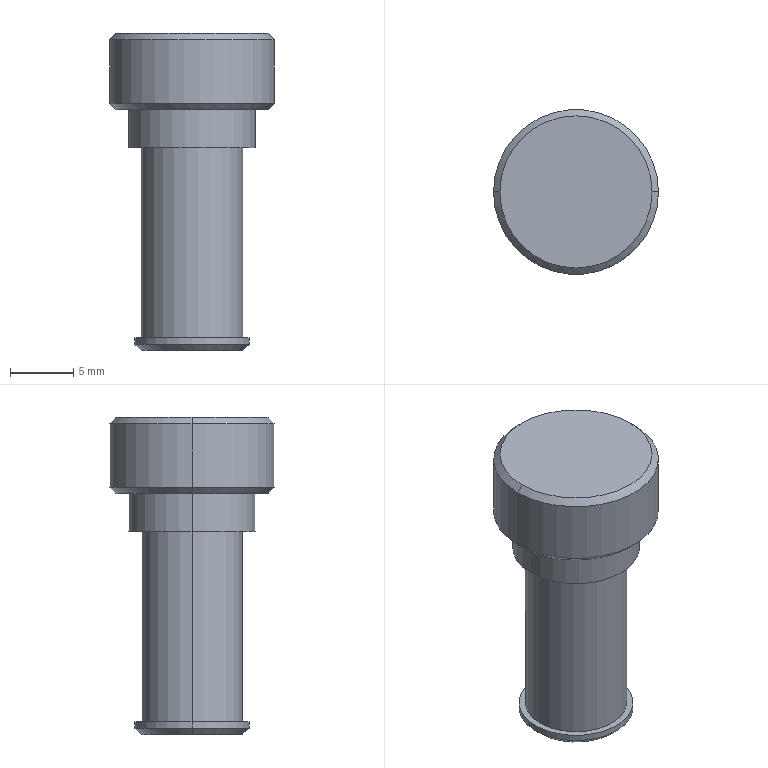Part | SolidWorks | features ICE 4, Chamfer 1, Extrusion 1 | 1 solid | 19 faces | box 13 x 13 x 25 mm | volume 1836 mm3 | cylinder 8 | cone 6 | plane 5 | commonest cylinder face diameters 8 x2 9 x2 10 x2 13 x2
STEP:
#1=CARTESIAN_POINT('',(-6.,0.,19.));
#2=VERTEX_POINT('',#1);
#3=CARTESIAN_POINT('',(6.,0.,19.));
#4=VERTEX_POINT('',#3);
#5=CARTESIAN_POINT('',(0.,0.,19.));
#6=DIRECTION('',(0.,0.,-1.));
#7=DIRECTION('',(1.,0.,0.));
#8=AXIS2_PLACEMENT_3D('',#5,#6,#7);
#9=CIRCLE('',#8,6.);
#10=EDGE_CURVE('',#2,#4,#9,.T.);
#11=ORIENTED_EDGE('',*,*,#10,.F.);
#12=CARTESIAN_POINT('',(-6.5,0.,19.5));
#13=VERTEX_POINT('',#12);
#14=CARTESIAN_POINT('',(-6.5,0.,19.5));
#15=DIRECTION('',(-0.7071,0.,0.7071));
#16=VECTOR('',#15,1000.);
#17=LINE('',#14,#16);
#18=EDGE_CURVE('',#2,#13,#17,.T.);
#19=ORIENTED_EDGE('',*,*,#18,.T.);
#20=CARTESIAN_POINT('',(6.5,0.,19.5));
#21=VERTEX_POINT('',#20);
#22=CARTESIAN_POINT('',(0.,0.,19.5));
#23=DIRECTION('',(0.,0.,1.));
#24=DIRECTION('',(1.,0.,0.));
#25=AXIS2_PLACEMENT_3D('',#22,#23,#24);
#26=CIRCLE('',#25,6.5);
#27=EDGE_CURVE('',#21,#13,#26,.T.);
#28=ORIENTED_EDGE('',*,*,#27,.F.);
#29=CARTESIAN_POINT('',(6.5,0.,19.5));
#30=DIRECTION('',(0.7071,0.,0.7071));
#31=VECTOR('',#30,1000.);
#32=LINE('',#29,#31);
#33=EDGE_CURVE('',#4,#21,#32,.T.);
#34=ORIENTED_EDGE('',*,*,#33,.F.);
#35=EDGE_LOOP('',(#11,#19,#28,#34));
#36=FACE_OUTER_BOUND('',#35,.T.);
#37=CARTESIAN_POINT('',(0.,0.,19.5));
#38=DIRECTION('',(0.,0.,1.));
#39=DIRECTION('',(1.,0.,0.));
#40=AXIS2_PLACEMENT_3D('',#37,#38,#39);
#41=CONICAL_SURFACE('',#40,6.5,0.7854);
#42=ADVANCED_FACE('',(#36),#41,.T.);
#43=CARTESIAN_POINT('',(-4.,0.,0.));
#44=VERTEX_POINT('',#43);
#45=CARTESIAN_POINT('',(4.,0.,0.));
#46=VERTEX_POINT('',#45);
#47=CARTESIAN_POINT('',(0.,0.,0.));
#48=DIRECTION('',(0.,0.,-1.));
#49=DIRECTION('',(1.,0.,0.));
#50=AXIS2_PLACEMENT_3D('',#47,#48,#49);
#51=CIRCLE('',#50,4.);
#52=EDGE_CURVE('',#44,#46,#51,.T.);
#53=ORIENTED_EDGE('',*,*,#52,.F.);
#54=CARTESIAN_POINT('',(-4.5,0.,0.5));
#55=VERTEX_POINT('',#54);
#56=CARTESIAN_POINT('',(-4.5,0.,0.5));
#57=DIRECTION('',(-0.7071,0.,0.7071));
#58=VECTOR('',#57,1000.);
#59=LINE('',#56,#58);
#60=EDGE_CURVE('',#44,#55,#59,.T.);
#61=ORIENTED_EDGE('',*,*,#60,.T.);
#62=CARTESIAN_POINT('',(4.5,0.,0.5));
#63=VERTEX_POINT('',#62);
#64=CARTESIAN_POINT('',(0.,0.,0.5));
#65=DIRECTION('',(0.,0.,1.));
#66=DIRECTION('',(1.,0.,0.));
#67=AXIS2_PLACEMENT_3D('',#64,#65,#66);
#68=CIRCLE('',#67,4.5);
#69=EDGE_CURVE('',#63,#55,#68,.T.);
#70=ORIENTED_EDGE('',*,*,#69,.F.);
#71=CARTESIAN_POINT('',(4.5,0.,0.5));
#72=DIRECTION('',(0.7071,0.,0.7071));
#73=VECTOR('',#72,1000.);
#74=LINE('',#71,#73);
#75=EDGE_CURVE('',#46,#63,#74,.T.);
#76=ORIENTED_EDGE('',*,*,#75,.F.);
#77=EDGE_LOOP('',(#53,#61,#70,#76));
#78=FACE_OUTER_BOUND('',#77,.T.);
#79=CARTESIAN_POINT('',(0.,0.,0.5));
#80=DIRECTION('',(0.,0.,1.));
#81=DIRECTION('',(1.,0.,0.));
#82=AXIS2_PLACEMENT_3D('',#79,#80,#81);
#83=CONICAL_SURFACE('',#82,4.5,0.7854);
#84=ADVANCED_FACE('',(#78),#83,.T.);
#85=CARTESIAN_POINT('',(6.,0.,25.));
#86=VERTEX_POINT('',#85);
#87=CARTESIAN_POINT('',(-6.,0.,25.));
#88=VERTEX_POINT('',#87);
#89=CARTESIAN_POINT('',(0.,0.,25.));
#90=DIRECTION('',(0.,0.,1.));
#91=DIRECTION('',(1.,0.,0.));
#92=AXIS2_PLACEMENT_3D('',#89,#90,#91);
#93=CIRCLE('',#92,6.);
#94=EDGE_CURVE('',#86,#88,#93,.T.);
#95=ORIENTED_EDGE('',*,*,#94,.F.);
#96=CARTESIAN_POINT('',(6.5,0.,24.5));
#97=VERTEX_POINT('',#96);
#98=CARTESIAN_POINT('',(6.,0.,25.));
#99=DIRECTION('',(0.7071,0.,-0.7071));
#100=VECTOR('',#99,1000.);
#101=LINE('',#98,#100);
#102=EDGE_CURVE('',#86,#97,#101,.T.);
#103=ORIENTED_EDGE('',*,*,#102,.T.);
#104=CARTESIAN_POINT('',(-6.5,0.,24.5));
#105=VERTEX_POINT('',#104);
#106=CARTESIAN_POINT('',(0.,0.,24.5));
#107=DIRECTION('',(0.,0.,-1.));
#108=DIRECTION('',(1.,0.,0.));
#109=AXIS2_PLACEMENT_3D('',#106,#107,#108);
#110=CIRCLE('',#109,6.5);
#111=EDGE_CURVE('',#105,#97,#110,.T.);
#112=ORIENTED_EDGE('',*,*,#111,.F.);
#113=CARTESIAN_POINT('',(-6.,0.,25.));
#114=DIRECTION('',(-0.7071,0.,-0.7071));
#115=VECTOR('',#114,1000.);
#116=LINE('',#113,#115);
#117=EDGE_CURVE('',#88,#105,#116,.T.);
#118=ORIENTED_EDGE('',*,*,#117,.F.);
#119=EDGE_LOOP('',(#95,#103,#112,#118));
#120=FACE_OUTER_BOUND('',#119,.T.);
#121=CARTESIAN_POINT('',(0.,0.,25.));
#122=DIRECTION('',(0.,0.,-1.));
#123=DIRECTION('',(-1.,0.,0.));
#124=AXIS2_PLACEMENT_3D('',#121,#122,#123);
#125=CONICAL_SURFACE('',#124,6.,0.7854);
#126=ADVANCED_FACE('',(#120),#125,.T.);
#127=ORIENTED_EDGE('',*,*,#111,.T.);
#128=CARTESIAN_POINT('',(6.5,0.,25.));
#129=DIRECTION('',(0.,0.,-1.));
#130=VECTOR('',#129,1000.);
#131=LINE('',#128,#130);
#132=EDGE_CURVE('',#97,#21,#131,.T.);
#133=ORIENTED_EDGE('',*,*,#132,.T.);
#134=ORIENTED_EDGE('',*,*,#27,.T.);
#135=CARTESIAN_POINT('',(-6.5,0.,25.));
#136=DIRECTION('',(0.,0.,-1.));
#137=VECTOR('',#136,1000.);
#138=LINE('',#135,#137);
#139=EDGE_CURVE('',#105,#13,#138,.T.);
#140=ORIENTED_EDGE('',*,*,#139,.F.);
#141=EDGE_LOOP('',(#127,#133,#134,#140));
#142=FACE_OUTER_BOUND('',#141,.T.);
#143=CARTESIAN_POINT('',(0.,0.,25.));
#144=DIRECTION('',(0.,0.,-1.));
#145=DIRECTION('',(-1.,0.,0.));
#146=AXIS2_PLACEMENT_3D('',#143,#144,#145);
#147=CYLINDRICAL_SURFACE('',#146,6.5);
#148=ADVANCED_FACE('',(#142),#147,.T.);
#149=CARTESIAN_POINT('',(5.,0.,19.));
#150=VERTEX_POINT('',#149);
#151=CARTESIAN_POINT('',(-5.,0.,19.));
#152=VERTEX_POINT('',#151);
#153=CARTESIAN_POINT('',(0.,0.,19.));
#154=DIRECTION('',(0.,0.,1.));
#155=DIRECTION('',(1.,0.,0.));
#156=AXIS2_PLACEMENT_3D('',#153,#154,#155);
#157=CIRCLE('',#156,5.);
#158=EDGE_CURVE('',#150,#152,#157,.T.);
#159=ORIENTED_EDGE('',*,*,#158,.F.);
#160=CARTESIAN_POINT('',(5.,0.,16.));
#161=VERTEX_POINT('',#160);
#162=CARTESIAN_POINT('',(5.,0.,19.));
#163=DIRECTION('',(0.,0.,-1.));
#164=VECTOR('',#163,1000.);
#165=LINE('',#162,#164);
#166=EDGE_CURVE('',#150,#161,#165,.T.);
#167=ORIENTED_EDGE('',*,*,#166,.T.);
#168=CARTESIAN_POINT('',(-5.,0.,16.));
#169=VERTEX_POINT('',#168);
#170=CARTESIAN_POINT('',(0.,0.,16.));
#171=DIRECTION('',(0.,0.,1.));
#172=DIRECTION('',(1.,0.,0.));
#173=AXIS2_PLACEMENT_3D('',#170,#171,#172);
#174=CIRCLE('',#173,5.);
#175=EDGE_CURVE('',#161,#169,#174,.T.);
#176=ORIENTED_EDGE('',*,*,#175,.T.);
#177=CARTESIAN_POINT('',(-5.,0.,19.));
#178=DIRECTION('',(0.,0.,-1.));
#179=VECTOR('',#178,1000.);
#180=LINE('',#177,#179);
#181=EDGE_CURVE('',#152,#169,#180,.T.);
#182=ORIENTED_EDGE('',*,*,#181,.F.);
#183=EDGE_LOOP('',(#159,#167,#176,#182));
#184=FACE_OUTER_BOUND('',#183,.T.);
#185=CARTESIAN_POINT('',(0.,0.,19.));
#186=DIRECTION('',(0.,0.,-1.));
#187=DIRECTION('',(-1.,0.,0.));
#188=AXIS2_PLACEMENT_3D('',#185,#186,#187);
#189=CYLINDRICAL_SURFACE('',#188,5.);
#190=ADVANCED_FACE('',(#184),#189,.T.);
#191=CARTESIAN_POINT('',(4.,0.,16.));
#192=VERTEX_POINT('',#191);
#193=CARTESIAN_POINT('',(-4.,0.,16.));
#194=VERTEX_POINT('',#193);
#195=CARTESIAN_POINT('',(0.,0.,16.));
#196=DIRECTION('',(0.,0.,1.));
#197=DIRECTION('',(1.,0.,0.));
#198=AXIS2_PLACEMENT_3D('',#195,#196,#197);
#199=CIRCLE('',#198,4.);
#200=EDGE_CURVE('',#192,#194,#199,.T.);
#201=ORIENTED_EDGE('',*,*,#200,.F.);
#202=CARTESIAN_POINT('',(4.,0.,1.));
#203=VERTEX_POINT('',#202);
#204=CARTESIAN_POINT('',(4.,0.,2.));
#205=DIRECTION('',(0.,0.,-1.));
#206=VECTOR('',#205,1000.);
#207=LINE('',#204,#206);
#208=EDGE_CURVE('',#192,#203,#207,.T.);
#209=ORIENTED_EDGE('',*,*,#208,.T.);
#210=CARTESIAN_POINT('',(-4.,0.,1.));
#211=VERTEX_POINT('',#210);
#212=CARTESIAN_POINT('',(0.,0.,1.));
#213=DIRECTION('',(0.,0.,1.));
#214=DIRECTION('',(1.,0.,0.));
#215=AXIS2_PLACEMENT_3D('',#212,#213,#214);
#216=CIRCLE('',#215,4.);
#217=EDGE_CURVE('',#203,#211,#216,.T.);
#218=ORIENTED_EDGE('',*,*,#217,.T.);
#219=CARTESIAN_POINT('',(-4.,0.,2.));
#220=DIRECTION('',(0.,0.,-1.));
#221=VECTOR('',#220,1000.);
#222=LINE('',#219,#221);
#223=EDGE_CURVE('',#194,#211,#222,.T.);
#224=ORIENTED_EDGE('',*,*,#223,.F.);
#225=EDGE_LOOP('',(#201,#209,#218,#224));
#226=FACE_OUTER_BOUND('',#225,.T.);
#227=CARTESIAN_POINT('',(0.,0.,2.));
#228=DIRECTION('',(0.,0.,-1.));
#229=DIRECTION('',(-1.,0.,0.));
#230=AXIS2_PLACEMENT_3D('',#227,#228,#229);
#231=CYLINDRICAL_SURFACE('',#230,4.);
#232=ADVANCED_FACE('',(#226),#231,.T.);
#233=CARTESIAN_POINT('',(4.5,0.,1.));
#234=VERTEX_POINT('',#233);
#235=CARTESIAN_POINT('',(-4.5,0.,1.));
#236=VERTEX_POINT('',#235);
#237=CARTESIAN_POINT('',(0.,0.,1.));
#238=DIRECTION('',(0.,0.,1.));
#239=DIRECTION('',(1.,0.,0.));
#240=AXIS2_PLACEMENT_3D('',#237,#238,#239);
#241=CIRCLE('',#240,4.5);
#242=EDGE_CURVE('',#234,#236,#241,.T.);
#243=ORIENTED_EDGE('',*,*,#242,.F.);
#244=CARTESIAN_POINT('',(4.5,0.,1.));
#245=DIRECTION('',(0.,0.,-1.));
#246=VECTOR('',#245,1000.);
#247=LINE('',#244,#246);
#248=EDGE_CURVE('',#234,#63,#247,.T.);
#249=ORIENTED_EDGE('',*,*,#248,.T.);
#250=ORIENTED_EDGE('',*,*,#69,.T.);
#251=CARTESIAN_POINT('',(-4.5,0.,1.));
#252=DIRECTION('',(0.,0.,-1.));
#253=VECTOR('',#252,1000.);
#254=LINE('',#251,#253);
#255=EDGE_CURVE('',#236,#55,#254,.T.);
#256=ORIENTED_EDGE('',*,*,#255,.F.);
#257=EDGE_LOOP('',(#243,#249,#250,#256));
#258=FACE_OUTER_BOUND('',#257,.T.);
#259=CARTESIAN_POINT('',(0.,0.,1.));
#260=DIRECTION('',(0.,0.,-1.));
#261=DIRECTION('',(-1.,0.,0.));
#262=AXIS2_PLACEMENT_3D('',#259,#260,#261);
#263=CYLINDRICAL_SURFACE('',#262,4.5);
#264=ADVANCED_FACE('',(#258),#263,.T.);
#265=ORIENTED_EDGE('',*,*,#248,.F.);
#266=CARTESIAN_POINT('',(0.,0.,1.));
#267=DIRECTION('',(0.,0.,1.));
#268=DIRECTION('',(1.,0.,0.));
#269=AXIS2_PLACEMENT_3D('',#266,#267,#268);
#270=CIRCLE('',#269,4.5);
#271=EDGE_CURVE('',#236,#234,#270,.T.);
#272=ORIENTED_EDGE('',*,*,#271,.F.);
#273=ORIENTED_EDGE('',*,*,#255,.T.);
#274=CARTESIAN_POINT('',(0.,0.,0.5));
#275=DIRECTION('',(0.,0.,1.));
#276=DIRECTION('',(1.,0.,0.));
#277=AXIS2_PLACEMENT_3D('',#274,#275,#276);
#278=CIRCLE('',#277,4.5);
#279=EDGE_CURVE('',#55,#63,#278,.T.);
#280=ORIENTED_EDGE('',*,*,#279,.T.);
#281=EDGE_LOOP('',(#265,#272,#273,#280));
#282=FACE_OUTER_BOUND('',#281,.T.);
#283=CARTESIAN_POINT('',(0.,0.,1.));
#284=DIRECTION('',(0.,0.,-1.));
#285=DIRECTION('',(-1.,0.,0.));
#286=AXIS2_PLACEMENT_3D('',#283,#284,#285);
#287=CYLINDRICAL_SURFACE('',#286,4.5);
#288=ADVANCED_FACE('',(#282),#287,.T.);
#289=CARTESIAN_POINT('',(0.,0.,1.));
#290=DIRECTION('',(0.,0.,1.));
#291=DIRECTION('',(1.,0.,0.));
#292=AXIS2_PLACEMENT_3D('',#289,#290,#291);
#293=CIRCLE('',#292,4.);
#294=EDGE_CURVE('',#211,#203,#293,.T.);
#295=ORIENTED_EDGE('',*,*,#294,.F.);
#296=ORIENTED_EDGE('',*,*,#217,.F.);
#297=EDGE_LOOP('',(#295,#296));
#298=FACE_BOUND('',#297,.T.);
#299=ORIENTED_EDGE('',*,*,#271,.T.);
#300=ORIENTED_EDGE('',*,*,#242,.T.);
#301=EDGE_LOOP('',(#299,#300));
#302=FACE_OUTER_BOUND('',#301,.T.);
#303=CARTESIAN_POINT('',(0.,0.,1.));
#304=DIRECTION('',(0.,0.,1.));
#305=DIRECTION('',(1.,0.,0.));
#306=AXIS2_PLACEMENT_3D('',#303,#304,#305);
#307=PLANE('',#306);
#308=ADVANCED_FACE('',(#298,#302),#307,.T.);
#309=CARTESIAN_POINT('',(0.,0.,0.));
#310=DIRECTION('',(0.,0.,-1.));
#311=DIRECTION('',(1.,0.,0.));
#312=AXIS2_PLACEMENT_3D('',#309,#310,#311);
#313=CIRCLE('',#312,4.);
#314=EDGE_CURVE('',#46,#44,#313,.T.);
#315=ORIENTED_EDGE('',*,*,#314,.T.);
#316=ORIENTED_EDGE('',*,*,#52,.T.);
#317=EDGE_LOOP('',(#315,#316));
#318=FACE_OUTER_BOUND('',#317,.T.);
#319=CARTESIAN_POINT('',(0.,0.,0.));
#320=DIRECTION('',(0.,0.,1.));
#321=DIRECTION('',(1.,0.,0.));
#322=AXIS2_PLACEMENT_3D('',#319,#320,#321);
#323=PLANE('',#322);
#324=ADVANCED_FACE('',(#318),#323,.F.);
#325=ORIENTED_EDGE('',*,*,#208,.F.);
#326=CARTESIAN_POINT('',(0.,0.,16.));
#327=DIRECTION('',(0.,0.,1.));
#328=DIRECTION('',(1.,0.,0.));
#329=AXIS2_PLACEMENT_3D('',#326,#327,#328);
#330=CIRCLE('',#329,4.);
#331=EDGE_CURVE('',#194,#192,#330,.T.);
#332=ORIENTED_EDGE('',*,*,#331,.F.);
#333=ORIENTED_EDGE('',*,*,#223,.T.);
#334=ORIENTED_EDGE('',*,*,#294,.T.);
#335=EDGE_LOOP('',(#325,#332,#333,#334));
#336=FACE_OUTER_BOUND('',#335,.T.);
#337=CARTESIAN_POINT('',(0.,0.,2.));
#338=DIRECTION('',(0.,0.,-1.));
#339=DIRECTION('',(-1.,0.,0.));
#340=AXIS2_PLACEMENT_3D('',#337,#338,#339);
#341=CYLINDRICAL_SURFACE('',#340,4.);
#342=ADVANCED_FACE('',(#336),#341,.T.);
#343=ORIENTED_EDGE('',*,*,#166,.F.);
#344=CARTESIAN_POINT('',(0.,0.,19.));
#345=DIRECTION('',(0.,0.,1.));
#346=DIRECTION('',(1.,0.,0.));
#347=AXIS2_PLACEMENT_3D('',#344,#345,#346);
#348=CIRCLE('',#347,5.);
#349=EDGE_CURVE('',#152,#150,#348,.T.);
#350=ORIENTED_EDGE('',*,*,#349,.F.);
#351=ORIENTED_EDGE('',*,*,#181,.T.);
#352=CARTESIAN_POINT('',(0.,0.,16.));
#353=DIRECTION('',(0.,0.,1.));
#354=DIRECTION('',(1.,0.,0.));
#355=AXIS2_PLACEMENT_3D('',#352,#353,#354);
#356=CIRCLE('',#355,5.);
#357=EDGE_CURVE('',#169,#161,#356,.T.);
#358=ORIENTED_EDGE('',*,*,#357,.T.);
#359=EDGE_LOOP('',(#343,#350,#351,#358));
#360=FACE_OUTER_BOUND('',#359,.T.);
#361=CARTESIAN_POINT('',(0.,0.,19.));
#362=DIRECTION('',(0.,0.,-1.));
#363=DIRECTION('',(-1.,0.,0.));
#364=AXIS2_PLACEMENT_3D('',#361,#362,#363);
#365=CYLINDRICAL_SURFACE('',#364,5.);
#366=ADVANCED_FACE('',(#360),#365,.T.);
#367=ORIENTED_EDGE('',*,*,#331,.T.);
#368=ORIENTED_EDGE('',*,*,#200,.T.);
#369=EDGE_LOOP('',(#367,#368));
#370=FACE_BOUND('',#369,.T.);
#371=ORIENTED_EDGE('',*,*,#357,.F.);
#372=ORIENTED_EDGE('',*,*,#175,.F.);
#373=EDGE_LOOP('',(#371,#372));
#374=FACE_OUTER_BOUND('',#373,.T.);
#375=CARTESIAN_POINT('',(0.,0.,16.));
#376=DIRECTION('',(0.,0.,1.));
#377=DIRECTION('',(1.,0.,0.));
#378=AXIS2_PLACEMENT_3D('',#375,#376,#377);
#379=PLANE('',#378);
#380=ADVANCED_FACE('',(#370,#374),#379,.F.);
#381=ORIENTED_EDGE('',*,*,#132,.F.);
#382=CARTESIAN_POINT('',(0.,0.,24.5));
#383=DIRECTION('',(0.,0.,-1.));
#384=DIRECTION('',(1.,0.,0.));
#385=AXIS2_PLACEMENT_3D('',#382,#383,#384);
#386=CIRCLE('',#385,6.5);
#387=EDGE_CURVE('',#97,#105,#386,.T.);
#388=ORIENTED_EDGE('',*,*,#387,.T.);
#389=ORIENTED_EDGE('',*,*,#139,.T.);
#390=CARTESIAN_POINT('',(0.,0.,19.5));
#391=DIRECTION('',(0.,0.,1.));
#392=DIRECTION('',(1.,0.,0.));
#393=AXIS2_PLACEMENT_3D('',#390,#391,#392);
#394=CIRCLE('',#393,6.5);
#395=EDGE_CURVE('',#13,#21,#394,.T.);
#396=ORIENTED_EDGE('',*,*,#395,.T.);
#397=EDGE_LOOP('',(#381,#388,#389,#396));
#398=FACE_OUTER_BOUND('',#397,.T.);
#399=CARTESIAN_POINT('',(0.,0.,25.));
#400=DIRECTION('',(0.,0.,-1.));
#401=DIRECTION('',(-1.,0.,0.));
#402=AXIS2_PLACEMENT_3D('',#399,#400,#401);
#403=CYLINDRICAL_SURFACE('',#402,6.5);
#404=ADVANCED_FACE('',(#398),#403,.T.);
#405=CARTESIAN_POINT('',(0.,0.,25.));
#406=DIRECTION('',(0.,0.,1.));
#407=DIRECTION('',(1.,0.,0.));
#408=AXIS2_PLACEMENT_3D('',#405,#406,#407);
#409=CIRCLE('',#408,6.);
#410=EDGE_CURVE('',#88,#86,#409,.T.);
#411=ORIENTED_EDGE('',*,*,#410,.T.);
#412=ORIENTED_EDGE('',*,*,#94,.T.);
#413=EDGE_LOOP('',(#411,#412));
#414=FACE_OUTER_BOUND('',#413,.T.);
#415=CARTESIAN_POINT('',(0.,0.,25.));
#416=DIRECTION('',(0.,0.,1.));
#417=DIRECTION('',(1.,0.,0.));
#418=AXIS2_PLACEMENT_3D('',#415,#416,#417);
#419=PLANE('',#418);
#420=ADVANCED_FACE('',(#414),#419,.T.);
#421=CARTESIAN_POINT('',(0.,0.,19.));
#422=DIRECTION('',(0.,0.,-1.));
#423=DIRECTION('',(1.,0.,0.));
#424=AXIS2_PLACEMENT_3D('',#421,#422,#423);
#425=CIRCLE('',#424,6.);
#426=EDGE_CURVE('',#4,#2,#425,.T.);
#427=ORIENTED_EDGE('',*,*,#426,.T.);
#428=ORIENTED_EDGE('',*,*,#10,.T.);
#429=EDGE_LOOP('',(#427,#428));
#430=FACE_OUTER_BOUND('',#429,.T.);
#431=ORIENTED_EDGE('',*,*,#349,.T.);
#432=ORIENTED_EDGE('',*,*,#158,.T.);
#433=EDGE_LOOP('',(#431,#432));
#434=FACE_BOUND('',#433,.T.);
#435=CARTESIAN_POINT('',(0.,0.,19.));
#436=DIRECTION('',(0.,0.,1.));
#437=DIRECTION('',(1.,0.,0.));
#438=AXIS2_PLACEMENT_3D('',#435,#436,#437);
#439=PLANE('',#438);
#440=ADVANCED_FACE('',(#430,#434),#439,.F.);
#441=ORIENTED_EDGE('',*,*,#102,.F.);
#442=ORIENTED_EDGE('',*,*,#410,.F.);
#443=ORIENTED_EDGE('',*,*,#117,.T.);
#444=ORIENTED_EDGE('',*,*,#387,.F.);
#445=EDGE_LOOP('',(#441,#442,#443,#444));
#446=FACE_OUTER_BOUND('',#445,.T.);
#447=CARTESIAN_POINT('',(0.,0.,25.));
#448=DIRECTION('',(0.,0.,-1.));
#449=DIRECTION('',(-1.,0.,0.));
#450=AXIS2_PLACEMENT_3D('',#447,#448,#449);
#451=CONICAL_SURFACE('',#450,6.,0.7854);
#452=ADVANCED_FACE('',(#446),#451,.T.);
#453=ORIENTED_EDGE('',*,*,#60,.F.);
#454=ORIENTED_EDGE('',*,*,#314,.F.);
#455=ORIENTED_EDGE('',*,*,#75,.T.);
#456=ORIENTED_EDGE('',*,*,#279,.F.);
#457=EDGE_LOOP('',(#453,#454,#455,#456));
#458=FACE_OUTER_BOUND('',#457,.T.);
#459=CARTESIAN_POINT('',(0.,0.,0.5));
#460=DIRECTION('',(0.,0.,1.));
#461=DIRECTION('',(1.,0.,0.));
#462=AXIS2_PLACEMENT_3D('',#459,#460,#461);
#463=CONICAL_SURFACE('',#462,4.5,0.7854);
#464=ADVANCED_FACE('',(#458),#463,.T.);
#465=ORIENTED_EDGE('',*,*,#18,.F.);
#466=ORIENTED_EDGE('',*,*,#426,.F.);
#467=ORIENTED_EDGE('',*,*,#33,.T.);
#468=ORIENTED_EDGE('',*,*,#395,.F.);
#469=EDGE_LOOP('',(#465,#466,#467,#468));
#470=FACE_OUTER_BOUND('',#469,.T.);
#471=CARTESIAN_POINT('',(0.,0.,19.5));
#472=DIRECTION('',(0.,0.,1.));
#473=DIRECTION('',(1.,0.,0.));
#474=AXIS2_PLACEMENT_3D('',#471,#472,#473);
#475=CONICAL_SURFACE('',#474,6.5,0.7854);
#476=ADVANCED_FACE('',(#470),#475,.T.);
#477=CLOSED_SHELL('',(#42,#84,#126,#148,#190,#232,#264,#288,#308,#324,#342,#366,#380,#404,#420,#440,#452,#464,#476));
#478=MANIFOLD_SOLID_BREP('',#477);
#479=CARTESIAN_POINT('',(0.,0.,0.));
#480=DIRECTION('',(0.,0.,1.));
#481=DIRECTION('',(1.,0.,0.));
#482=AXIS2_PLACEMENT_3D('',#479,#480,#481);
#483=(LENGTH_UNIT()NAMED_UNIT(*)SI_UNIT(.MILLI.,.METRE.));
#484=UNCERTAINTY_MEASURE_WITH_UNIT(LENGTH_MEASURE(0.00001),#483,'','');
#485=(NAMED_UNIT(*)PLANE_ANGLE_UNIT()SI_UNIT($,.RADIAN.));
#486=(NAMED_UNIT(*)SI_UNIT($,.STERADIAN.)SOLID_ANGLE_UNIT());
#487=(GEOMETRIC_REPRESENTATION_CONTEXT(3)GLOBAL_UNCERTAINTY_ASSIGNED_CONTEXT((#484))GLOBAL_UNIT_ASSIGNED_CONTEXT((#483,#485,#486))REPRESENTATION_CONTEXT('',''));
#488=ADVANCED_BREP_SHAPE_REPRESENTATION('',(#478,#482),#487);